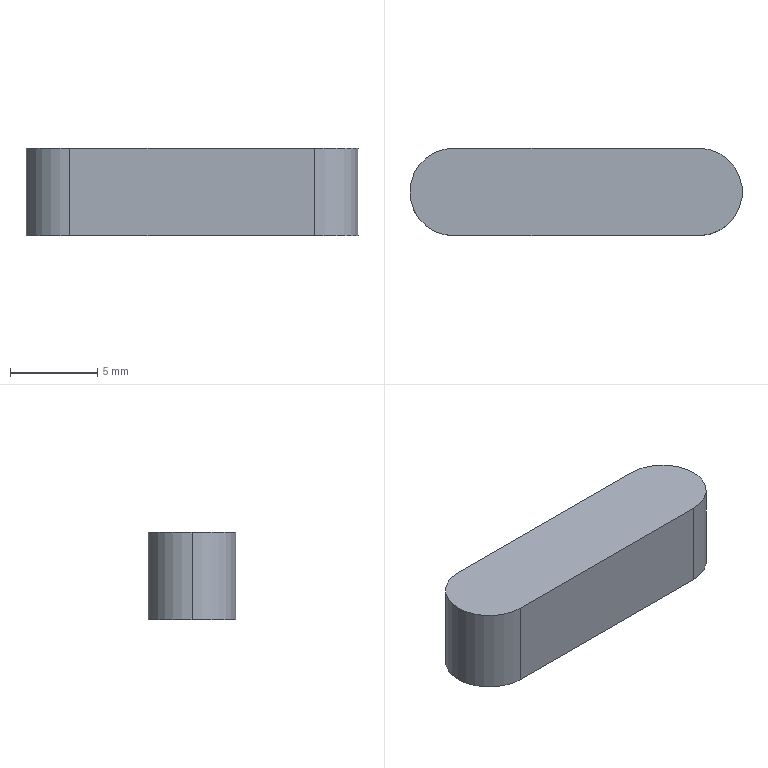Part | SolidWorks | features BaseBody 1 | 1 solid | 7 faces | box 19 x 5 x 5 mm | volume 448.175 mm3 | plane 4 | cylinder 3 | commonest cylinder face diameters 5 x3
STEP:
#1=CARTESIAN_POINT('',(-9.5,0.,5.));
#2=VERTEX_POINT('',#1);
#3=CARTESIAN_POINT('',(-7.,-2.5,5.));
#4=VERTEX_POINT('',#3);
#5=CARTESIAN_POINT('',(-7.,0.,5.));
#6=DIRECTION('',(0.,0.,1.));
#7=DIRECTION('',(1.,0.,0.));
#8=AXIS2_PLACEMENT_3D('',#5,#6,#7);
#9=CIRCLE('',#8,2.5);
#10=EDGE_CURVE('',#2,#4,#9,.T.);
#11=ORIENTED_EDGE('',*,*,#10,.F.);
#12=CARTESIAN_POINT('',(-9.5,0.,0.));
#13=VERTEX_POINT('',#12);
#14=CARTESIAN_POINT('',(-9.5,0.,5.));
#15=DIRECTION('',(0.,0.,-1.));
#16=VECTOR('',#15,1000.);
#17=LINE('',#14,#16);
#18=EDGE_CURVE('',#2,#13,#17,.T.);
#19=ORIENTED_EDGE('',*,*,#18,.T.);
#20=CARTESIAN_POINT('',(-7.,-2.5,0.));
#21=VERTEX_POINT('',#20);
#22=CARTESIAN_POINT('',(-7.,0.,0.));
#23=DIRECTION('',(0.,0.,1.));
#24=DIRECTION('',(1.,0.,0.));
#25=AXIS2_PLACEMENT_3D('',#22,#23,#24);
#26=CIRCLE('',#25,2.5);
#27=EDGE_CURVE('',#13,#21,#26,.T.);
#28=ORIENTED_EDGE('',*,*,#27,.T.);
#29=CARTESIAN_POINT('',(-7.,-2.5,5.));
#30=DIRECTION('',(0.,0.,-1.));
#31=VECTOR('',#30,1000.);
#32=LINE('',#29,#31);
#33=EDGE_CURVE('',#4,#21,#32,.T.);
#34=ORIENTED_EDGE('',*,*,#33,.F.);
#35=EDGE_LOOP('',(#11,#19,#28,#34));
#36=FACE_OUTER_BOUND('',#35,.T.);
#37=CARTESIAN_POINT('',(-7.,0.,5.));
#38=DIRECTION('',(0.,0.,-1.));
#39=DIRECTION('',(-1.,0.,0.));
#40=AXIS2_PLACEMENT_3D('',#37,#38,#39);
#41=CYLINDRICAL_SURFACE('',#40,2.5);
#42=ADVANCED_FACE('',(#36),#41,.T.);
#43=CARTESIAN_POINT('',(-7.,2.5,0.));
#44=VERTEX_POINT('',#43);
#45=CARTESIAN_POINT('',(-7.,0.,0.));
#46=DIRECTION('',(0.,0.,1.));
#47=DIRECTION('',(1.,0.,0.));
#48=AXIS2_PLACEMENT_3D('',#45,#46,#47);
#49=CIRCLE('',#48,2.5);
#50=EDGE_CURVE('',#44,#13,#49,.T.);
#51=ORIENTED_EDGE('',*,*,#50,.F.);
#52=CARTESIAN_POINT('',(7.,2.5,0.));
#53=VERTEX_POINT('',#52);
#54=CARTESIAN_POINT('',(-7.,2.5,0.));
#55=DIRECTION('',(-1.,0.,0.));
#56=VECTOR('',#55,1000.);
#57=LINE('',#54,#56);
#58=EDGE_CURVE('',#53,#44,#57,.T.);
#59=ORIENTED_EDGE('',*,*,#58,.F.);
#60=CARTESIAN_POINT('',(7.,-2.5,0.));
#61=VERTEX_POINT('',#60);
#62=CARTESIAN_POINT('',(7.,0.,0.));
#63=DIRECTION('',(0.,0.,1.));
#64=DIRECTION('',(1.,0.,0.));
#65=AXIS2_PLACEMENT_3D('',#62,#63,#64);
#66=CIRCLE('',#65,2.5);
#67=EDGE_CURVE('',#61,#53,#66,.T.);
#68=ORIENTED_EDGE('',*,*,#67,.F.);
#69=CARTESIAN_POINT('',(-7.,-2.5,0.));
#70=DIRECTION('',(1.,0.,0.));
#71=VECTOR('',#70,1000.);
#72=LINE('',#69,#71);
#73=EDGE_CURVE('',#21,#61,#72,.T.);
#74=ORIENTED_EDGE('',*,*,#73,.F.);
#75=ORIENTED_EDGE('',*,*,#27,.F.);
#76=EDGE_LOOP('',(#51,#59,#68,#74,#75));
#77=FACE_OUTER_BOUND('',#76,.T.);
#78=CARTESIAN_POINT('',(-7.,0.,0.));
#79=DIRECTION('',(0.,0.,1.));
#80=DIRECTION('',(1.,0.,0.));
#81=AXIS2_PLACEMENT_3D('',#78,#79,#80);
#82=PLANE('',#81);
#83=ADVANCED_FACE('',(#77),#82,.F.);
#84=CARTESIAN_POINT('',(7.,2.5,5.));
#85=VERTEX_POINT('',#84);
#86=CARTESIAN_POINT('',(-7.,2.5,5.));
#87=VERTEX_POINT('',#86);
#88=CARTESIAN_POINT('',(-7.,2.5,5.));
#89=DIRECTION('',(-1.,0.,0.));
#90=VECTOR('',#89,1000.);
#91=LINE('',#88,#90);
#92=EDGE_CURVE('',#85,#87,#91,.T.);
#93=ORIENTED_EDGE('',*,*,#92,.T.);
#94=CARTESIAN_POINT('',(-7.,0.,5.));
#95=DIRECTION('',(0.,0.,1.));
#96=DIRECTION('',(1.,0.,0.));
#97=AXIS2_PLACEMENT_3D('',#94,#95,#96);
#98=CIRCLE('',#97,2.5);
#99=EDGE_CURVE('',#87,#2,#98,.T.);
#100=ORIENTED_EDGE('',*,*,#99,.T.);
#101=ORIENTED_EDGE('',*,*,#10,.T.);
#102=CARTESIAN_POINT('',(7.,-2.5,5.));
#103=VERTEX_POINT('',#102);
#104=CARTESIAN_POINT('',(-7.,-2.5,5.));
#105=DIRECTION('',(1.,0.,0.));
#106=VECTOR('',#105,1000.);
#107=LINE('',#104,#106);
#108=EDGE_CURVE('',#4,#103,#107,.T.);
#109=ORIENTED_EDGE('',*,*,#108,.T.);
#110=CARTESIAN_POINT('',(7.,0.,5.));
#111=DIRECTION('',(0.,0.,1.));
#112=DIRECTION('',(1.,0.,0.));
#113=AXIS2_PLACEMENT_3D('',#110,#111,#112);
#114=CIRCLE('',#113,2.5);
#115=EDGE_CURVE('',#103,#85,#114,.T.);
#116=ORIENTED_EDGE('',*,*,#115,.T.);
#117=EDGE_LOOP('',(#93,#100,#101,#109,#116));
#118=FACE_OUTER_BOUND('',#117,.T.);
#119=CARTESIAN_POINT('',(-7.,0.,5.));
#120=DIRECTION('',(0.,0.,1.));
#121=DIRECTION('',(1.,0.,0.));
#122=AXIS2_PLACEMENT_3D('',#119,#120,#121);
#123=PLANE('',#122);
#124=ADVANCED_FACE('',(#118),#123,.T.);
#125=ORIENTED_EDGE('',*,*,#58,.T.);
#126=CARTESIAN_POINT('',(-7.,2.5,5.));
#127=DIRECTION('',(0.,0.,-1.));
#128=VECTOR('',#127,1000.);
#129=LINE('',#126,#128);
#130=EDGE_CURVE('',#87,#44,#129,.T.);
#131=ORIENTED_EDGE('',*,*,#130,.F.);
#132=ORIENTED_EDGE('',*,*,#92,.F.);
#133=CARTESIAN_POINT('',(7.,2.5,5.));
#134=DIRECTION('',(0.,0.,-1.));
#135=VECTOR('',#134,1000.);
#136=LINE('',#133,#135);
#137=EDGE_CURVE('',#85,#53,#136,.T.);
#138=ORIENTED_EDGE('',*,*,#137,.T.);
#139=EDGE_LOOP('',(#125,#131,#132,#138));
#140=FACE_OUTER_BOUND('',#139,.T.);
#141=CARTESIAN_POINT('',(-7.,2.5,5.));
#142=DIRECTION('',(0.,-1.,0.));
#143=DIRECTION('',(0.,0.,-1.));
#144=AXIS2_PLACEMENT_3D('',#141,#142,#143);
#145=PLANE('',#144);
#146=ADVANCED_FACE('',(#140),#145,.F.);
#147=ORIENTED_EDGE('',*,*,#67,.T.);
#148=ORIENTED_EDGE('',*,*,#137,.F.);
#149=ORIENTED_EDGE('',*,*,#115,.F.);
#150=CARTESIAN_POINT('',(7.,-2.5,5.));
#151=DIRECTION('',(0.,0.,-1.));
#152=VECTOR('',#151,1000.);
#153=LINE('',#150,#152);
#154=EDGE_CURVE('',#103,#61,#153,.T.);
#155=ORIENTED_EDGE('',*,*,#154,.T.);
#156=EDGE_LOOP('',(#147,#148,#149,#155));
#157=FACE_OUTER_BOUND('',#156,.T.);
#158=CARTESIAN_POINT('',(7.,0.,5.));
#159=DIRECTION('',(0.,0.,-1.));
#160=DIRECTION('',(-1.,0.,0.));
#161=AXIS2_PLACEMENT_3D('',#158,#159,#160);
#162=CYLINDRICAL_SURFACE('',#161,2.5);
#163=ADVANCED_FACE('',(#157),#162,.T.);
#164=ORIENTED_EDGE('',*,*,#73,.T.);
#165=ORIENTED_EDGE('',*,*,#154,.F.);
#166=ORIENTED_EDGE('',*,*,#108,.F.);
#167=ORIENTED_EDGE('',*,*,#33,.T.);
#168=EDGE_LOOP('',(#164,#165,#166,#167));
#169=FACE_OUTER_BOUND('',#168,.T.);
#170=CARTESIAN_POINT('',(-7.,-2.5,5.));
#171=DIRECTION('',(0.,1.,0.));
#172=DIRECTION('',(1.,0.,0.));
#173=AXIS2_PLACEMENT_3D('',#170,#171,#172);
#174=PLANE('',#173);
#175=ADVANCED_FACE('',(#169),#174,.F.);
#176=ORIENTED_EDGE('',*,*,#18,.F.);
#177=ORIENTED_EDGE('',*,*,#99,.F.);
#178=ORIENTED_EDGE('',*,*,#130,.T.);
#179=ORIENTED_EDGE('',*,*,#50,.T.);
#180=EDGE_LOOP('',(#176,#177,#178,#179));
#181=FACE_OUTER_BOUND('',#180,.T.);
#182=CARTESIAN_POINT('',(-7.,0.,5.));
#183=DIRECTION('',(0.,0.,-1.));
#184=DIRECTION('',(-1.,0.,0.));
#185=AXIS2_PLACEMENT_3D('',#182,#183,#184);
#186=CYLINDRICAL_SURFACE('',#185,2.5);
#187=ADVANCED_FACE('',(#181),#186,.T.);
#188=CLOSED_SHELL('',(#42,#83,#124,#146,#163,#175,#187));
#189=MANIFOLD_SOLID_BREP('',#188);
#190=CARTESIAN_POINT('',(0.,0.,0.));
#191=DIRECTION('',(0.,0.,1.));
#192=DIRECTION('',(1.,0.,0.));
#193=AXIS2_PLACEMENT_3D('',#190,#191,#192);
#194=(LENGTH_UNIT()NAMED_UNIT(*)SI_UNIT(.MILLI.,.METRE.));
#195=UNCERTAINTY_MEASURE_WITH_UNIT(LENGTH_MEASURE(0.00001),#194,'','');
#196=(NAMED_UNIT(*)PLANE_ANGLE_UNIT()SI_UNIT($,.RADIAN.));
#197=(NAMED_UNIT(*)SI_UNIT($,.STERADIAN.)SOLID_ANGLE_UNIT());
#198=(GEOMETRIC_REPRESENTATION_CONTEXT(3)GLOBAL_UNCERTAINTY_ASSIGNED_CONTEXT((#195))GLOBAL_UNIT_ASSIGNED_CONTEXT((#194,#196,#197))REPRESENTATION_CONTEXT('',''));
#199=ADVANCED_BREP_SHAPE_REPRESENTATION('',(#189,#193),#198);